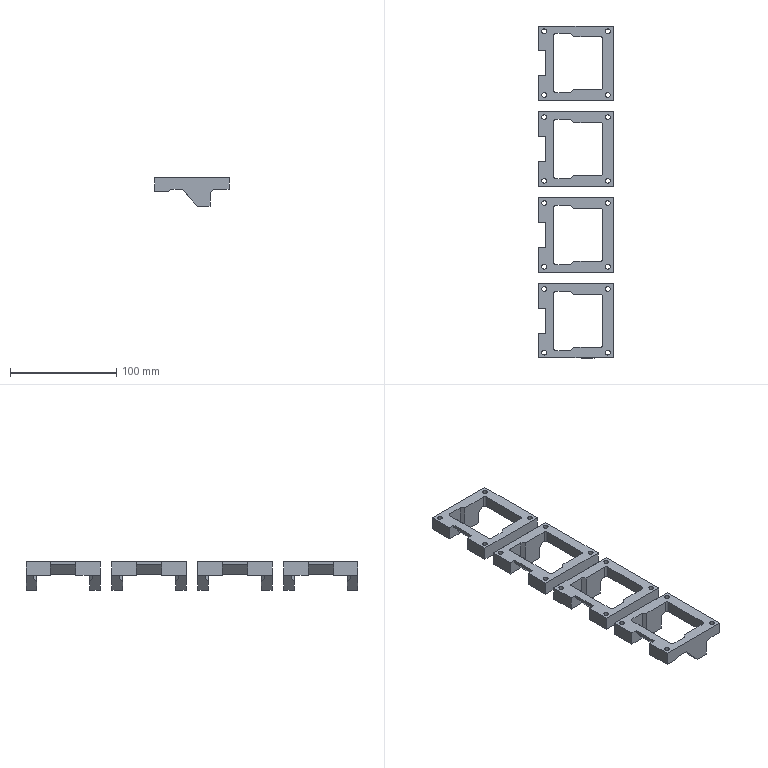Part | 4 solids | 200 faces | box 70 x 313 x 26.9 mm | volume 126662 mm3 | plane 128 | cylinder 56 | cone 16 | commonest cylinder face diameters 4.5 x32 4 x16 10 x8